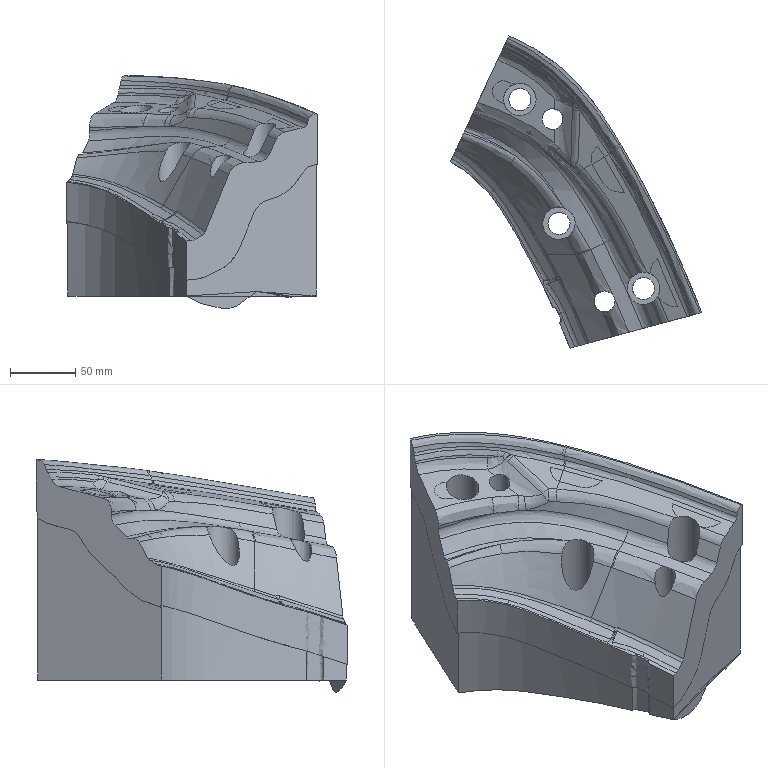Part | NX | features solid 2 | 1 solid | 107 faces | volume 2467833 mm3 | spline 88 | cylinder 10 | plane 9 | commonest cylinder face diameters 25 x5 17 x3 16 x2